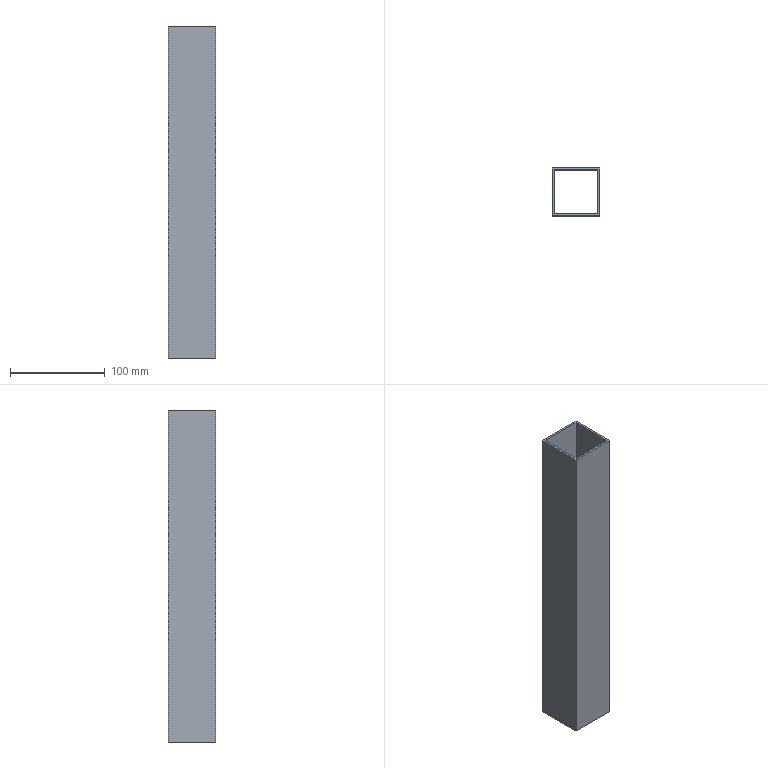Part | SolidWorks | features Extrusion 1 | 1 solid | 10 faces | box 50 x 50 x 350 mm | volume 134400 mm3 | plane 10
STEP:
#1=CARTESIAN_POINT('',(25.,-25.,350.));
#2=VERTEX_POINT('',#1);
#3=CARTESIAN_POINT('',(25.,25.,350.));
#4=VERTEX_POINT('',#3);
#5=CARTESIAN_POINT('',(25.,-25.,350.));
#6=DIRECTION('',(0.,1.,0.));
#7=VECTOR('',#6,1000.);
#8=LINE('',#5,#7);
#9=EDGE_CURVE('',#2,#4,#8,.T.);
#10=ORIENTED_EDGE('',*,*,#9,.T.);
#11=CARTESIAN_POINT('',(-25.,25.,350.));
#12=VERTEX_POINT('',#11);
#13=CARTESIAN_POINT('',(-25.,25.,350.));
#14=DIRECTION('',(-1.,0.,0.));
#15=VECTOR('',#14,1000.);
#16=LINE('',#13,#15);
#17=EDGE_CURVE('',#4,#12,#16,.T.);
#18=ORIENTED_EDGE('',*,*,#17,.T.);
#19=CARTESIAN_POINT('',(-25.,-25.,350.));
#20=VERTEX_POINT('',#19);
#21=CARTESIAN_POINT('',(-25.,-25.,350.));
#22=DIRECTION('',(0.,-1.,0.));
#23=VECTOR('',#22,1000.);
#24=LINE('',#21,#23);
#25=EDGE_CURVE('',#12,#20,#24,.T.);
#26=ORIENTED_EDGE('',*,*,#25,.T.);
#27=CARTESIAN_POINT('',(-25.,-25.,350.));
#28=DIRECTION('',(1.,0.,0.));
#29=VECTOR('',#28,1000.);
#30=LINE('',#27,#29);
#31=EDGE_CURVE('',#20,#2,#30,.T.);
#32=ORIENTED_EDGE('',*,*,#31,.T.);
#33=EDGE_LOOP('',(#10,#18,#26,#32));
#34=FACE_OUTER_BOUND('',#33,.T.);
#35=CARTESIAN_POINT('',(23.,-23.,350.));
#36=VERTEX_POINT('',#35);
#37=CARTESIAN_POINT('',(23.,23.,350.));
#38=VERTEX_POINT('',#37);
#39=CARTESIAN_POINT('',(23.,-23.,350.));
#40=DIRECTION('',(0.,1.,0.));
#41=VECTOR('',#40,1000.);
#42=LINE('',#39,#41);
#43=EDGE_CURVE('',#36,#38,#42,.T.);
#44=ORIENTED_EDGE('',*,*,#43,.F.);
#45=CARTESIAN_POINT('',(-23.,-23.,350.));
#46=VERTEX_POINT('',#45);
#47=CARTESIAN_POINT('',(-23.,-23.,350.));
#48=DIRECTION('',(1.,0.,0.));
#49=VECTOR('',#48,1000.);
#50=LINE('',#47,#49);
#51=EDGE_CURVE('',#46,#36,#50,.T.);
#52=ORIENTED_EDGE('',*,*,#51,.F.);
#53=CARTESIAN_POINT('',(-23.,23.,350.));
#54=VERTEX_POINT('',#53);
#55=CARTESIAN_POINT('',(-23.,-23.,350.));
#56=DIRECTION('',(0.,-1.,0.));
#57=VECTOR('',#56,1000.);
#58=LINE('',#55,#57);
#59=EDGE_CURVE('',#54,#46,#58,.T.);
#60=ORIENTED_EDGE('',*,*,#59,.F.);
#61=CARTESIAN_POINT('',(-23.,23.,350.));
#62=DIRECTION('',(-1.,0.,0.));
#63=VECTOR('',#62,1000.);
#64=LINE('',#61,#63);
#65=EDGE_CURVE('',#38,#54,#64,.T.);
#66=ORIENTED_EDGE('',*,*,#65,.F.);
#67=EDGE_LOOP('',(#44,#52,#60,#66));
#68=FACE_BOUND('',#67,.T.);
#69=CARTESIAN_POINT('',(0.,0.,350.));
#70=DIRECTION('',(0.,0.,-1.));
#71=DIRECTION('',(-1.,0.,0.));
#72=AXIS2_PLACEMENT_3D('',#69,#70,#71);
#73=PLANE('',#72);
#74=ADVANCED_FACE('',(#34,#68),#73,.F.);
#75=CARTESIAN_POINT('',(25.,-25.,0.));
#76=VERTEX_POINT('',#75);
#77=CARTESIAN_POINT('',(25.,25.,0.));
#78=VERTEX_POINT('',#77);
#79=CARTESIAN_POINT('',(25.,-25.,0.));
#80=DIRECTION('',(0.,1.,0.));
#81=VECTOR('',#80,1000.);
#82=LINE('',#79,#81);
#83=EDGE_CURVE('',#76,#78,#82,.T.);
#84=ORIENTED_EDGE('',*,*,#83,.F.);
#85=CARTESIAN_POINT('',(-25.,-25.,0.));
#86=VERTEX_POINT('',#85);
#87=CARTESIAN_POINT('',(-25.,-25.,0.));
#88=DIRECTION('',(1.,0.,0.));
#89=VECTOR('',#88,1000.);
#90=LINE('',#87,#89);
#91=EDGE_CURVE('',#86,#76,#90,.T.);
#92=ORIENTED_EDGE('',*,*,#91,.F.);
#93=CARTESIAN_POINT('',(-25.,25.,0.));
#94=VERTEX_POINT('',#93);
#95=CARTESIAN_POINT('',(-25.,-25.,0.));
#96=DIRECTION('',(0.,-1.,0.));
#97=VECTOR('',#96,1000.);
#98=LINE('',#95,#97);
#99=EDGE_CURVE('',#94,#86,#98,.T.);
#100=ORIENTED_EDGE('',*,*,#99,.F.);
#101=CARTESIAN_POINT('',(-25.,25.,0.));
#102=DIRECTION('',(-1.,0.,0.));
#103=VECTOR('',#102,1000.);
#104=LINE('',#101,#103);
#105=EDGE_CURVE('',#78,#94,#104,.T.);
#106=ORIENTED_EDGE('',*,*,#105,.F.);
#107=EDGE_LOOP('',(#84,#92,#100,#106));
#108=FACE_OUTER_BOUND('',#107,.T.);
#109=CARTESIAN_POINT('',(-23.,-23.,0.));
#110=VERTEX_POINT('',#109);
#111=CARTESIAN_POINT('',(23.,-23.,0.));
#112=VERTEX_POINT('',#111);
#113=CARTESIAN_POINT('',(-23.,-23.,0.));
#114=DIRECTION('',(1.,0.,0.));
#115=VECTOR('',#114,1000.);
#116=LINE('',#113,#115);
#117=EDGE_CURVE('',#110,#112,#116,.T.);
#118=ORIENTED_EDGE('',*,*,#117,.T.);
#119=CARTESIAN_POINT('',(23.,23.,0.));
#120=VERTEX_POINT('',#119);
#121=CARTESIAN_POINT('',(23.,-23.,0.));
#122=DIRECTION('',(0.,1.,0.));
#123=VECTOR('',#122,1000.);
#124=LINE('',#121,#123);
#125=EDGE_CURVE('',#112,#120,#124,.T.);
#126=ORIENTED_EDGE('',*,*,#125,.T.);
#127=CARTESIAN_POINT('',(-23.,23.,0.));
#128=VERTEX_POINT('',#127);
#129=CARTESIAN_POINT('',(-23.,23.,0.));
#130=DIRECTION('',(-1.,0.,0.));
#131=VECTOR('',#130,1000.);
#132=LINE('',#129,#131);
#133=EDGE_CURVE('',#120,#128,#132,.T.);
#134=ORIENTED_EDGE('',*,*,#133,.T.);
#135=CARTESIAN_POINT('',(-23.,-23.,0.));
#136=DIRECTION('',(0.,-1.,0.));
#137=VECTOR('',#136,1000.);
#138=LINE('',#135,#137);
#139=EDGE_CURVE('',#128,#110,#138,.T.);
#140=ORIENTED_EDGE('',*,*,#139,.T.);
#141=EDGE_LOOP('',(#118,#126,#134,#140));
#142=FACE_BOUND('',#141,.T.);
#143=CARTESIAN_POINT('',(0.,0.,0.));
#144=DIRECTION('',(0.,0.,-1.));
#145=DIRECTION('',(-1.,0.,0.));
#146=AXIS2_PLACEMENT_3D('',#143,#144,#145);
#147=PLANE('',#146);
#148=ADVANCED_FACE('',(#108,#142),#147,.T.);
#149=ORIENTED_EDGE('',*,*,#83,.T.);
#150=CARTESIAN_POINT('',(25.,25.,350.));
#151=DIRECTION('',(0.,0.,-1.));
#152=VECTOR('',#151,1000.);
#153=LINE('',#150,#152);
#154=EDGE_CURVE('',#4,#78,#153,.T.);
#155=ORIENTED_EDGE('',*,*,#154,.F.);
#156=ORIENTED_EDGE('',*,*,#9,.F.);
#157=CARTESIAN_POINT('',(25.,-25.,350.));
#158=DIRECTION('',(0.,0.,-1.));
#159=VECTOR('',#158,1000.);
#160=LINE('',#157,#159);
#161=EDGE_CURVE('',#2,#76,#160,.T.);
#162=ORIENTED_EDGE('',*,*,#161,.T.);
#163=EDGE_LOOP('',(#149,#155,#156,#162));
#164=FACE_OUTER_BOUND('',#163,.T.);
#165=CARTESIAN_POINT('',(25.,-25.,350.));
#166=DIRECTION('',(-1.,0.,0.));
#167=DIRECTION('',(0.,0.,1.));
#168=AXIS2_PLACEMENT_3D('',#165,#166,#167);
#169=PLANE('',#168);
#170=ADVANCED_FACE('',(#164),#169,.F.);
#171=ORIENTED_EDGE('',*,*,#105,.T.);
#172=CARTESIAN_POINT('',(-25.,25.,350.));
#173=DIRECTION('',(0.,0.,-1.));
#174=VECTOR('',#173,1000.);
#175=LINE('',#172,#174);
#176=EDGE_CURVE('',#12,#94,#175,.T.);
#177=ORIENTED_EDGE('',*,*,#176,.F.);
#178=ORIENTED_EDGE('',*,*,#17,.F.);
#179=ORIENTED_EDGE('',*,*,#154,.T.);
#180=EDGE_LOOP('',(#171,#177,#178,#179));
#181=FACE_OUTER_BOUND('',#180,.T.);
#182=CARTESIAN_POINT('',(-25.,25.,350.));
#183=DIRECTION('',(0.,-1.,0.));
#184=DIRECTION('',(0.,0.,-1.));
#185=AXIS2_PLACEMENT_3D('',#182,#183,#184);
#186=PLANE('',#185);
#187=ADVANCED_FACE('',(#181),#186,.F.);
#188=ORIENTED_EDGE('',*,*,#99,.T.);
#189=CARTESIAN_POINT('',(-25.,-25.,350.));
#190=DIRECTION('',(0.,0.,-1.));
#191=VECTOR('',#190,1000.);
#192=LINE('',#189,#191);
#193=EDGE_CURVE('',#20,#86,#192,.T.);
#194=ORIENTED_EDGE('',*,*,#193,.F.);
#195=ORIENTED_EDGE('',*,*,#25,.F.);
#196=ORIENTED_EDGE('',*,*,#176,.T.);
#197=EDGE_LOOP('',(#188,#194,#195,#196));
#198=FACE_OUTER_BOUND('',#197,.T.);
#199=CARTESIAN_POINT('',(-25.,-25.,350.));
#200=DIRECTION('',(1.,0.,0.));
#201=DIRECTION('',(0.,0.,-1.));
#202=AXIS2_PLACEMENT_3D('',#199,#200,#201);
#203=PLANE('',#202);
#204=ADVANCED_FACE('',(#198),#203,.F.);
#205=ORIENTED_EDGE('',*,*,#91,.T.);
#206=ORIENTED_EDGE('',*,*,#161,.F.);
#207=ORIENTED_EDGE('',*,*,#31,.F.);
#208=ORIENTED_EDGE('',*,*,#193,.T.);
#209=EDGE_LOOP('',(#205,#206,#207,#208));
#210=FACE_OUTER_BOUND('',#209,.T.);
#211=CARTESIAN_POINT('',(-25.,-25.,350.));
#212=DIRECTION('',(0.,1.,0.));
#213=DIRECTION('',(0.,0.,1.));
#214=AXIS2_PLACEMENT_3D('',#211,#212,#213);
#215=PLANE('',#214);
#216=ADVANCED_FACE('',(#210),#215,.F.);
#217=ORIENTED_EDGE('',*,*,#125,.F.);
#218=CARTESIAN_POINT('',(23.,-23.,350.));
#219=DIRECTION('',(0.,0.,-1.));
#220=VECTOR('',#219,1000.);
#221=LINE('',#218,#220);
#222=EDGE_CURVE('',#36,#112,#221,.T.);
#223=ORIENTED_EDGE('',*,*,#222,.F.);
#224=ORIENTED_EDGE('',*,*,#43,.T.);
#225=CARTESIAN_POINT('',(23.,23.,350.));
#226=DIRECTION('',(0.,0.,-1.));
#227=VECTOR('',#226,1000.);
#228=LINE('',#225,#227);
#229=EDGE_CURVE('',#38,#120,#228,.T.);
#230=ORIENTED_EDGE('',*,*,#229,.T.);
#231=EDGE_LOOP('',(#217,#223,#224,#230));
#232=FACE_OUTER_BOUND('',#231,.T.);
#233=CARTESIAN_POINT('',(23.,-23.,350.));
#234=DIRECTION('',(-1.,0.,0.));
#235=DIRECTION('',(0.,0.,1.));
#236=AXIS2_PLACEMENT_3D('',#233,#234,#235);
#237=PLANE('',#236);
#238=ADVANCED_FACE('',(#232),#237,.T.);
#239=ORIENTED_EDGE('',*,*,#133,.F.);
#240=ORIENTED_EDGE('',*,*,#229,.F.);
#241=ORIENTED_EDGE('',*,*,#65,.T.);
#242=CARTESIAN_POINT('',(-23.,23.,350.));
#243=DIRECTION('',(0.,0.,-1.));
#244=VECTOR('',#243,1000.);
#245=LINE('',#242,#244);
#246=EDGE_CURVE('',#54,#128,#245,.T.);
#247=ORIENTED_EDGE('',*,*,#246,.T.);
#248=EDGE_LOOP('',(#239,#240,#241,#247));
#249=FACE_OUTER_BOUND('',#248,.T.);
#250=CARTESIAN_POINT('',(-23.,23.,350.));
#251=DIRECTION('',(0.,-1.,0.));
#252=DIRECTION('',(0.,0.,-1.));
#253=AXIS2_PLACEMENT_3D('',#250,#251,#252);
#254=PLANE('',#253);
#255=ADVANCED_FACE('',(#249),#254,.T.);
#256=ORIENTED_EDGE('',*,*,#139,.F.);
#257=ORIENTED_EDGE('',*,*,#246,.F.);
#258=ORIENTED_EDGE('',*,*,#59,.T.);
#259=CARTESIAN_POINT('',(-23.,-23.,350.));
#260=DIRECTION('',(0.,0.,-1.));
#261=VECTOR('',#260,1000.);
#262=LINE('',#259,#261);
#263=EDGE_CURVE('',#46,#110,#262,.T.);
#264=ORIENTED_EDGE('',*,*,#263,.T.);
#265=EDGE_LOOP('',(#256,#257,#258,#264));
#266=FACE_OUTER_BOUND('',#265,.T.);
#267=CARTESIAN_POINT('',(-23.,-23.,350.));
#268=DIRECTION('',(1.,0.,0.));
#269=DIRECTION('',(0.,0.,-1.));
#270=AXIS2_PLACEMENT_3D('',#267,#268,#269);
#271=PLANE('',#270);
#272=ADVANCED_FACE('',(#266),#271,.T.);
#273=ORIENTED_EDGE('',*,*,#117,.F.);
#274=ORIENTED_EDGE('',*,*,#263,.F.);
#275=ORIENTED_EDGE('',*,*,#51,.T.);
#276=ORIENTED_EDGE('',*,*,#222,.T.);
#277=EDGE_LOOP('',(#273,#274,#275,#276));
#278=FACE_OUTER_BOUND('',#277,.T.);
#279=CARTESIAN_POINT('',(-23.,-23.,350.));
#280=DIRECTION('',(0.,1.,0.));
#281=DIRECTION('',(0.,0.,1.));
#282=AXIS2_PLACEMENT_3D('',#279,#280,#281);
#283=PLANE('',#282);
#284=ADVANCED_FACE('',(#278),#283,.T.);
#285=CLOSED_SHELL('',(#74,#148,#170,#187,#204,#216,#238,#255,#272,#284));
#286=MANIFOLD_SOLID_BREP('',#285);
#287=CARTESIAN_POINT('',(0.,0.,0.));
#288=DIRECTION('',(0.,0.,1.));
#289=DIRECTION('',(1.,0.,0.));
#290=AXIS2_PLACEMENT_3D('',#287,#288,#289);
#291=(LENGTH_UNIT()NAMED_UNIT(*)SI_UNIT(.MILLI.,.METRE.));
#292=UNCERTAINTY_MEASURE_WITH_UNIT(LENGTH_MEASURE(0.00001),#291,'','');
#293=(NAMED_UNIT(*)PLANE_ANGLE_UNIT()SI_UNIT($,.RADIAN.));
#294=(NAMED_UNIT(*)SI_UNIT($,.STERADIAN.)SOLID_ANGLE_UNIT());
#295=(GEOMETRIC_REPRESENTATION_CONTEXT(3)GLOBAL_UNCERTAINTY_ASSIGNED_CONTEXT((#292))GLOBAL_UNIT_ASSIGNED_CONTEXT((#291,#293,#294))REPRESENTATION_CONTEXT('',''));
#296=ADVANCED_BREP_SHAPE_REPRESENTATION('',(#286,#290),#295);